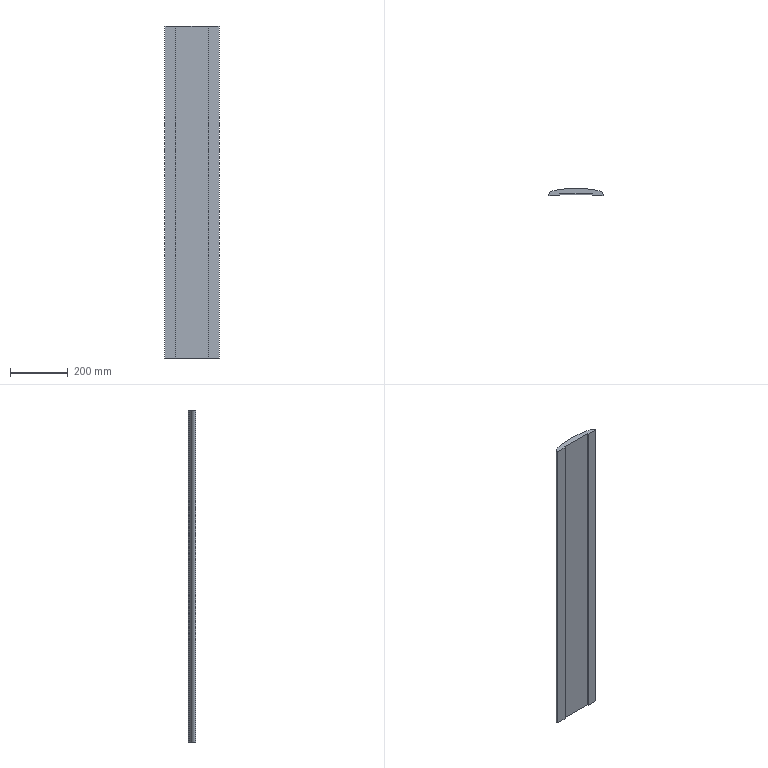Part | SolidWorks | features Extrusion 1, Fillet 1 | 1 solid | 31 faces | box 188.037 x 25 x 1150 mm | volume 3794355 mm3 | cylinder 24 | plane 7 | commonest cylinder face diameters 0.2 x8 0.6 x6 661 x5 28 x3 0.4 x2
STEP:
#1=CARTESIAN_POINT('',(-94.018,0.7177,575.));
#2=VERTEX_POINT('',#1);
#3=CARTESIAN_POINT('',(-94.012,0.2909,575.));
#4=VERTEX_POINT('',#3);
#5=CARTESIAN_POINT('',(-80.018,0.7177,575.));
#6=DIRECTION('',(0.,0.,1.));
#7=DIRECTION('',(1.,0.,0.));
#8=AXIS2_PLACEMENT_3D('',#5,#6,#7);
#9=CIRCLE('',#8,14.);
#10=EDGE_CURVE('',#2,#4,#9,.T.);
#11=ORIENTED_EDGE('',*,*,#10,.F.);
#12=CARTESIAN_POINT('',(-94.018,0.7177,-575.));
#13=VERTEX_POINT('',#12);
#14=CARTESIAN_POINT('',(-94.018,0.7177,575.));
#15=DIRECTION('',(0.,0.,-1.));
#16=VECTOR('',#15,1000.);
#17=LINE('',#14,#16);
#18=EDGE_CURVE('',#2,#13,#17,.T.);
#19=ORIENTED_EDGE('',*,*,#18,.T.);
#20=CARTESIAN_POINT('',(-94.012,0.2909,-575.));
#21=VERTEX_POINT('',#20);
#22=CARTESIAN_POINT('',(-80.018,0.7177,-575.));
#23=DIRECTION('',(0.,0.,1.));
#24=DIRECTION('',(1.,0.,0.));
#25=AXIS2_PLACEMENT_3D('',#22,#23,#24);
#26=CIRCLE('',#25,14.);
#27=EDGE_CURVE('',#13,#21,#26,.T.);
#28=ORIENTED_EDGE('',*,*,#27,.T.);
#29=CARTESIAN_POINT('',(-94.012,0.2909,575.));
#30=DIRECTION('',(0.,0.,1.));
#31=VECTOR('',#30,1000.);
#32=LINE('',#29,#31);
#33=EDGE_CURVE('',#21,#4,#32,.T.);
#34=ORIENTED_EDGE('',*,*,#33,.T.);
#35=EDGE_LOOP('',(#11,#19,#28,#34));
#36=FACE_OUTER_BOUND('',#35,.T.);
#37=CARTESIAN_POINT('',(-80.018,0.7177,575.));
#38=DIRECTION('',(0.,0.,-1.));
#39=DIRECTION('',(-1.,0.,0.));
#40=AXIS2_PLACEMENT_3D('',#37,#38,#39);
#41=CYLINDRICAL_SURFACE('',#40,14.);
#42=ADVANCED_FACE('',(#36),#41,.T.);
#43=ORIENTED_EDGE('',*,*,#18,.F.);
#44=CARTESIAN_POINT('',(-83.558,14.263,575.));
#45=VERTEX_POINT('',#44);
#46=CARTESIAN_POINT('',(-80.018,0.7177,575.));
#47=DIRECTION('',(0.,0.,1.));
#48=DIRECTION('',(1.,0.,0.));
#49=AXIS2_PLACEMENT_3D('',#46,#47,#48);
#50=CIRCLE('',#49,14.);
#51=EDGE_CURVE('',#45,#2,#50,.T.);
#52=ORIENTED_EDGE('',*,*,#51,.F.);
#53=CARTESIAN_POINT('',(-83.558,14.263,-575.));
#54=VERTEX_POINT('',#53);
#55=CARTESIAN_POINT('',(-83.558,14.263,575.));
#56=DIRECTION('',(0.,0.,-1.));
#57=VECTOR('',#56,1000.);
#58=LINE('',#55,#57);
#59=EDGE_CURVE('',#45,#54,#58,.T.);
#60=ORIENTED_EDGE('',*,*,#59,.T.);
#61=CARTESIAN_POINT('',(-80.018,0.7177,-575.));
#62=DIRECTION('',(0.,0.,1.));
#63=DIRECTION('',(1.,0.,0.));
#64=AXIS2_PLACEMENT_3D('',#61,#62,#63);
#65=CIRCLE('',#64,14.);
#66=EDGE_CURVE('',#54,#13,#65,.T.);
#67=ORIENTED_EDGE('',*,*,#66,.T.);
#68=EDGE_LOOP('',(#43,#52,#60,#67));
#69=FACE_OUTER_BOUND('',#68,.T.);
#70=CARTESIAN_POINT('',(-80.018,0.7177,575.));
#71=DIRECTION('',(0.,0.,-1.));
#72=DIRECTION('',(-1.,0.,0.));
#73=AXIS2_PLACEMENT_3D('',#70,#71,#72);
#74=CYLINDRICAL_SURFACE('',#73,14.);
#75=ADVANCED_FACE('',(#69),#74,.T.);
#76=CARTESIAN_POINT('',(-93.712,0.,575.));
#77=VERTEX_POINT('',#76);
#78=CARTESIAN_POINT('',(-56.7,0.,575.));
#79=VERTEX_POINT('',#78);
#80=CARTESIAN_POINT('',(-56.7,0.,575.));
#81=DIRECTION('',(1.,0.,0.));
#82=VECTOR('',#81,1000.);
#83=LINE('',#80,#82);
#84=EDGE_CURVE('',#77,#79,#83,.T.);
#85=ORIENTED_EDGE('',*,*,#84,.F.);
#86=CARTESIAN_POINT('',(-93.712,0.,-575.));
#87=VERTEX_POINT('',#86);
#88=CARTESIAN_POINT('',(-93.712,0.,575.));
#89=DIRECTION('',(0.,0.,-1.));
#90=VECTOR('',#89,1000.);
#91=LINE('',#88,#90);
#92=EDGE_CURVE('',#77,#87,#91,.T.);
#93=ORIENTED_EDGE('',*,*,#92,.T.);
#94=CARTESIAN_POINT('',(-56.7,0.,-575.));
#95=VERTEX_POINT('',#94);
#96=CARTESIAN_POINT('',(-56.7,0.,-575.));
#97=DIRECTION('',(1.,0.,0.));
#98=VECTOR('',#97,1000.);
#99=LINE('',#96,#98);
#100=EDGE_CURVE('',#87,#95,#99,.T.);
#101=ORIENTED_EDGE('',*,*,#100,.T.);
#102=CARTESIAN_POINT('',(-56.7,0.,575.));
#103=DIRECTION('',(0.,0.,-1.));
#104=VECTOR('',#103,1000.);
#105=LINE('',#102,#104);
#106=EDGE_CURVE('',#79,#95,#105,.T.);
#107=ORIENTED_EDGE('',*,*,#106,.F.);
#108=EDGE_LOOP('',(#85,#93,#101,#107));
#109=FACE_OUTER_BOUND('',#108,.T.);
#110=CARTESIAN_POINT('',(-56.7,0.,575.));
#111=DIRECTION('',(0.,1.,0.));
#112=DIRECTION('',(-1.,0.,0.));
#113=AXIS2_PLACEMENT_3D('',#110,#111,#112);
#114=PLANE('',#113);
#115=ADVANCED_FACE('',(#109),#114,.F.);
#116=CARTESIAN_POINT('',(-56.5,0.2,-575.));
#117=VERTEX_POINT('',#116);
#118=CARTESIAN_POINT('',(-56.7,0.2,-575.));
#119=DIRECTION('',(0.,0.,1.));
#120=DIRECTION('',(-1.,0.,0.));
#121=AXIS2_PLACEMENT_3D('',#118,#119,#120);
#122=CIRCLE('',#121,0.2);
#123=EDGE_CURVE('',#95,#117,#122,.T.);
#124=ORIENTED_EDGE('',*,*,#123,.T.);
#125=CARTESIAN_POINT('',(-56.5,0.2,575.));
#126=VERTEX_POINT('',#125);
#127=CARTESIAN_POINT('',(-56.5,0.2,575.));
#128=DIRECTION('',(0.,0.,-1.));
#129=VECTOR('',#128,1000.);
#130=LINE('',#127,#129);
#131=EDGE_CURVE('',#126,#117,#130,.T.);
#132=ORIENTED_EDGE('',*,*,#131,.F.);
#133=CARTESIAN_POINT('',(-56.7,0.2,575.));
#134=DIRECTION('',(0.,0.,1.));
#135=DIRECTION('',(-1.,0.,0.));
#136=AXIS2_PLACEMENT_3D('',#133,#134,#135);
#137=CIRCLE('',#136,0.2);
#138=EDGE_CURVE('',#79,#126,#137,.T.);
#139=ORIENTED_EDGE('',*,*,#138,.F.);
#140=ORIENTED_EDGE('',*,*,#106,.T.);
#141=EDGE_LOOP('',(#124,#132,#139,#140));
#142=FACE_OUTER_BOUND('',#141,.T.);
#143=CARTESIAN_POINT('',(-56.7,0.2,575.));
#144=DIRECTION('',(0.,0.,-1.));
#145=DIRECTION('',(-1.,0.,0.));
#146=AXIS2_PLACEMENT_3D('',#143,#144,#145);
#147=CYLINDRICAL_SURFACE('',#146,0.2);
#148=ADVANCED_FACE('',(#142),#147,.T.);
#149=CARTESIAN_POINT('',(-56.5,4.5,-575.));
#150=VERTEX_POINT('',#149);
#151=CARTESIAN_POINT('',(-56.5,0.2,-575.));
#152=DIRECTION('',(0.,1.,0.));
#153=VECTOR('',#152,1000.);
#154=LINE('',#151,#153);
#155=EDGE_CURVE('',#117,#150,#154,.T.);
#156=ORIENTED_EDGE('',*,*,#155,.T.);
#157=CARTESIAN_POINT('',(-56.5,4.5,575.));
#158=VERTEX_POINT('',#157);
#159=CARTESIAN_POINT('',(-56.5,4.5,575.));
#160=DIRECTION('',(0.,0.,-1.));
#161=VECTOR('',#160,1000.);
#162=LINE('',#159,#161);
#163=EDGE_CURVE('',#158,#150,#162,.T.);
#164=ORIENTED_EDGE('',*,*,#163,.F.);
#165=CARTESIAN_POINT('',(-56.5,0.2,575.));
#166=DIRECTION('',(0.,1.,0.));
#167=VECTOR('',#166,1000.);
#168=LINE('',#165,#167);
#169=EDGE_CURVE('',#126,#158,#168,.T.);
#170=ORIENTED_EDGE('',*,*,#169,.F.);
#171=ORIENTED_EDGE('',*,*,#131,.T.);
#172=EDGE_LOOP('',(#156,#164,#170,#171));
#173=FACE_OUTER_BOUND('',#172,.T.);
#174=CARTESIAN_POINT('',(-56.5,0.2,575.));
#175=DIRECTION('',(-1.,0.,0.));
#176=DIRECTION('',(0.,-1.,0.));
#177=AXIS2_PLACEMENT_3D('',#174,#175,#176);
#178=PLANE('',#177);
#179=ADVANCED_FACE('',(#173),#178,.F.);
#180=CARTESIAN_POINT('',(56.5,4.5,-575.));
#181=VERTEX_POINT('',#180);
#182=CARTESIAN_POINT('',(-56.5,4.5,-575.));
#183=DIRECTION('',(1.,0.,0.));
#184=VECTOR('',#183,1000.);
#185=LINE('',#182,#184);
#186=EDGE_CURVE('',#150,#181,#185,.T.);
#187=ORIENTED_EDGE('',*,*,#186,.T.);
#188=CARTESIAN_POINT('',(56.5,4.5,575.));
#189=VERTEX_POINT('',#188);
#190=CARTESIAN_POINT('',(56.5,4.5,575.));
#191=DIRECTION('',(0.,0.,-1.));
#192=VECTOR('',#191,1000.);
#193=LINE('',#190,#192);
#194=EDGE_CURVE('',#189,#181,#193,.T.);
#195=ORIENTED_EDGE('',*,*,#194,.F.);
#196=CARTESIAN_POINT('',(-56.5,4.5,575.));
#197=DIRECTION('',(1.,0.,0.));
#198=VECTOR('',#197,1000.);
#199=LINE('',#196,#198);
#200=EDGE_CURVE('',#158,#189,#199,.T.);
#201=ORIENTED_EDGE('',*,*,#200,.F.);
#202=ORIENTED_EDGE('',*,*,#163,.T.);
#203=EDGE_LOOP('',(#187,#195,#201,#202));
#204=FACE_OUTER_BOUND('',#203,.T.);
#205=CARTESIAN_POINT('',(-56.5,4.5,575.));
#206=DIRECTION('',(0.,1.,0.));
#207=DIRECTION('',(-1.,0.,0.));
#208=AXIS2_PLACEMENT_3D('',#205,#206,#207);
#209=PLANE('',#208);
#210=ADVANCED_FACE('',(#204),#209,.F.);
#211=CARTESIAN_POINT('',(56.5,0.2,-575.));
#212=VERTEX_POINT('',#211);
#213=CARTESIAN_POINT('',(56.5,0.2,-575.));
#214=DIRECTION('',(0.,-1.,0.));
#215=VECTOR('',#214,1000.);
#216=LINE('',#213,#215);
#217=EDGE_CURVE('',#181,#212,#216,.T.);
#218=ORIENTED_EDGE('',*,*,#217,.T.);
#219=CARTESIAN_POINT('',(56.5,0.2,575.));
#220=VERTEX_POINT('',#219);
#221=CARTESIAN_POINT('',(56.5,0.2,575.));
#222=DIRECTION('',(0.,0.,-1.));
#223=VECTOR('',#222,1000.);
#224=LINE('',#221,#223);
#225=EDGE_CURVE('',#220,#212,#224,.T.);
#226=ORIENTED_EDGE('',*,*,#225,.F.);
#227=CARTESIAN_POINT('',(56.5,0.2,575.));
#228=DIRECTION('',(0.,-1.,0.));
#229=VECTOR('',#228,1000.);
#230=LINE('',#227,#229);
#231=EDGE_CURVE('',#189,#220,#230,.T.);
#232=ORIENTED_EDGE('',*,*,#231,.F.);
#233=ORIENTED_EDGE('',*,*,#194,.T.);
#234=EDGE_LOOP('',(#218,#226,#232,#233));
#235=FACE_OUTER_BOUND('',#234,.T.);
#236=CARTESIAN_POINT('',(56.5,0.2,575.));
#237=DIRECTION('',(1.,0.,0.));
#238=DIRECTION('',(0.,1.,0.));
#239=AXIS2_PLACEMENT_3D('',#236,#237,#238);
#240=PLANE('',#239);
#241=ADVANCED_FACE('',(#235),#240,.F.);
#242=CARTESIAN_POINT('',(56.7,0.,-575.));
#243=VERTEX_POINT('',#242);
#244=CARTESIAN_POINT('',(56.7,0.2,-575.));
#245=DIRECTION('',(0.,0.,1.));
#246=DIRECTION('',(-1.,0.,0.));
#247=AXIS2_PLACEMENT_3D('',#244,#245,#246);
#248=CIRCLE('',#247,0.2);
#249=EDGE_CURVE('',#212,#243,#248,.T.);
#250=ORIENTED_EDGE('',*,*,#249,.T.);
#251=CARTESIAN_POINT('',(56.7,0.,575.));
#252=VERTEX_POINT('',#251);
#253=CARTESIAN_POINT('',(56.7,0.,575.));
#254=DIRECTION('',(0.,0.,-1.));
#255=VECTOR('',#254,1000.);
#256=LINE('',#253,#255);
#257=EDGE_CURVE('',#252,#243,#256,.T.);
#258=ORIENTED_EDGE('',*,*,#257,.F.);
#259=CARTESIAN_POINT('',(56.7,0.2,575.));
#260=DIRECTION('',(0.,0.,1.));
#261=DIRECTION('',(-1.,0.,0.));
#262=AXIS2_PLACEMENT_3D('',#259,#260,#261);
#263=CIRCLE('',#262,0.2);
#264=EDGE_CURVE('',#220,#252,#263,.T.);
#265=ORIENTED_EDGE('',*,*,#264,.F.);
#266=ORIENTED_EDGE('',*,*,#225,.T.);
#267=EDGE_LOOP('',(#250,#258,#265,#266));
#268=FACE_OUTER_BOUND('',#267,.T.);
#269=CARTESIAN_POINT('',(56.7,0.2,575.));
#270=DIRECTION('',(0.,0.,-1.));
#271=DIRECTION('',(-1.,0.,0.));
#272=AXIS2_PLACEMENT_3D('',#269,#270,#271);
#273=CYLINDRICAL_SURFACE('',#272,0.2);
#274=ADVANCED_FACE('',(#268),#273,.T.);
#275=CARTESIAN_POINT('',(93.712,0.,-575.));
#276=VERTEX_POINT('',#275);
#277=CARTESIAN_POINT('',(94.,0.,-575.));
#278=DIRECTION('',(1.,0.,0.));
#279=VECTOR('',#278,1000.);
#280=LINE('',#277,#279);
#281=EDGE_CURVE('',#243,#276,#280,.T.);
#282=ORIENTED_EDGE('',*,*,#281,.T.);
#283=CARTESIAN_POINT('',(93.712,0.,575.));
#284=VERTEX_POINT('',#283);
#285=CARTESIAN_POINT('',(93.712,0.,575.));
#286=DIRECTION('',(0.,0.,1.));
#287=VECTOR('',#286,1000.);
#288=LINE('',#285,#287);
#289=EDGE_CURVE('',#276,#284,#288,.T.);
#290=ORIENTED_EDGE('',*,*,#289,.T.);
#291=CARTESIAN_POINT('',(94.,0.,575.));
#292=DIRECTION('',(1.,0.,0.));
#293=VECTOR('',#292,1000.);
#294=LINE('',#291,#293);
#295=EDGE_CURVE('',#252,#284,#294,.T.);
#296=ORIENTED_EDGE('',*,*,#295,.F.);
#297=ORIENTED_EDGE('',*,*,#257,.T.);
#298=EDGE_LOOP('',(#282,#290,#296,#297));
#299=FACE_OUTER_BOUND('',#298,.T.);
#300=CARTESIAN_POINT('',(94.,0.,575.));
#301=DIRECTION('',(0.,1.,0.));
#302=DIRECTION('',(-1.,0.,0.));
#303=AXIS2_PLACEMENT_3D('',#300,#301,#302);
#304=PLANE('',#303);
#305=ADVANCED_FACE('',(#299),#304,.F.);
#306=CARTESIAN_POINT('',(94.012,0.2909,575.));
#307=VERTEX_POINT('',#306);
#308=CARTESIAN_POINT('',(83.558,14.263,575.));
#309=VERTEX_POINT('',#308);
#310=CARTESIAN_POINT('',(80.018,0.7177,575.));
#311=DIRECTION('',(0.,0.,1.));
#312=DIRECTION('',(-1.,0.,0.));
#313=AXIS2_PLACEMENT_3D('',#310,#311,#312);
#314=CIRCLE('',#313,14.);
#315=EDGE_CURVE('',#307,#309,#314,.T.);
#316=ORIENTED_EDGE('',*,*,#315,.F.);
#317=CARTESIAN_POINT('',(94.012,0.2909,-575.));
#318=VERTEX_POINT('',#317);
#319=CARTESIAN_POINT('',(94.012,0.2909,575.));
#320=DIRECTION('',(0.,0.,-1.));
#321=VECTOR('',#320,1000.);
#322=LINE('',#319,#321);
#323=EDGE_CURVE('',#307,#318,#322,.T.);
#324=ORIENTED_EDGE('',*,*,#323,.T.);
#325=CARTESIAN_POINT('',(83.558,14.263,-575.));
#326=VERTEX_POINT('',#325);
#327=CARTESIAN_POINT('',(80.018,0.7177,-575.));
#328=DIRECTION('',(0.,0.,1.));
#329=DIRECTION('',(-1.,0.,0.));
#330=AXIS2_PLACEMENT_3D('',#327,#328,#329);
#331=CIRCLE('',#330,14.);
#332=EDGE_CURVE('',#318,#326,#331,.T.);
#333=ORIENTED_EDGE('',*,*,#332,.T.);
#334=CARTESIAN_POINT('',(83.558,14.263,575.));
#335=DIRECTION('',(0.,0.,-1.));
#336=VECTOR('',#335,1000.);
#337=LINE('',#334,#336);
#338=EDGE_CURVE('',#309,#326,#337,.T.);
#339=ORIENTED_EDGE('',*,*,#338,.F.);
#340=EDGE_LOOP('',(#316,#324,#333,#339));
#341=FACE_OUTER_BOUND('',#340,.T.);
#342=CARTESIAN_POINT('',(80.018,0.7177,575.));
#343=DIRECTION('',(0.,0.,-1.));
#344=DIRECTION('',(-1.,0.,0.));
#345=AXIS2_PLACEMENT_3D('',#342,#343,#344);
#346=CYLINDRICAL_SURFACE('',#345,14.);
#347=ADVANCED_FACE('',(#341),#346,.T.);
#348=CARTESIAN_POINT('',(60.381,19.438,-575.));
#349=VERTEX_POINT('',#348);
#350=CARTESIAN_POINT('',(0.,-305.5,-575.));
#351=DIRECTION('',(0.,0.,1.));
#352=DIRECTION('',(1.,0.,0.));
#353=AXIS2_PLACEMENT_3D('',#350,#351,#352);
#354=CIRCLE('',#353,330.5);
#355=EDGE_CURVE('',#326,#349,#354,.T.);
#356=ORIENTED_EDGE('',*,*,#355,.T.);
#357=CARTESIAN_POINT('',(60.381,19.438,575.));
#358=VERTEX_POINT('',#357);
#359=CARTESIAN_POINT('',(60.381,19.438,575.));
#360=DIRECTION('',(0.,0.,-1.));
#361=VECTOR('',#360,1000.);
#362=LINE('',#359,#361);
#363=EDGE_CURVE('',#358,#349,#362,.T.);
#364=ORIENTED_EDGE('',*,*,#363,.F.);
#365=CARTESIAN_POINT('',(0.,-305.5,575.));
#366=DIRECTION('',(0.,0.,1.));
#367=DIRECTION('',(1.,0.,0.));
#368=AXIS2_PLACEMENT_3D('',#365,#366,#367);
#369=CIRCLE('',#368,330.5);
#370=EDGE_CURVE('',#309,#358,#369,.T.);
#371=ORIENTED_EDGE('',*,*,#370,.F.);
#372=ORIENTED_EDGE('',*,*,#338,.T.);
#373=EDGE_LOOP('',(#356,#364,#371,#372));
#374=FACE_OUTER_BOUND('',#373,.T.);
#375=CARTESIAN_POINT('',(0.,-305.5,575.));
#376=DIRECTION('',(0.,0.,-1.));
#377=DIRECTION('',(-1.,0.,0.));
#378=AXIS2_PLACEMENT_3D('',#375,#376,#377);
#379=CYLINDRICAL_SURFACE('',#378,330.5);
#380=ADVANCED_FACE('',(#374),#379,.T.);
#381=CARTESIAN_POINT('',(60.272,19.381,-575.));
#382=VERTEX_POINT('',#381);
#383=CARTESIAN_POINT('',(60.363,19.339,-575.));
#384=DIRECTION('',(0.,0.,1.));
#385=DIRECTION('',(1.,0.,0.));
#386=AXIS2_PLACEMENT_3D('',#383,#384,#385);
#387=CIRCLE('',#386,0.1);
#388=EDGE_CURVE('',#349,#382,#387,.T.);
#389=ORIENTED_EDGE('',*,*,#388,.T.);
#390=CARTESIAN_POINT('',(60.272,19.381,575.));
#391=VERTEX_POINT('',#390);
#392=CARTESIAN_POINT('',(60.272,19.381,575.));
#393=DIRECTION('',(0.,0.,-1.));
#394=VECTOR('',#393,1000.);
#395=LINE('',#392,#394);
#396=EDGE_CURVE('',#391,#382,#395,.T.);
#397=ORIENTED_EDGE('',*,*,#396,.F.);
#398=CARTESIAN_POINT('',(60.363,19.339,575.));
#399=DIRECTION('',(0.,0.,1.));
#400=DIRECTION('',(1.,0.,0.));
#401=AXIS2_PLACEMENT_3D('',#398,#399,#400);
#402=CIRCLE('',#401,0.1);
#403=EDGE_CURVE('',#358,#391,#402,.T.);
#404=ORIENTED_EDGE('',*,*,#403,.F.);
#405=ORIENTED_EDGE('',*,*,#363,.T.);
#406=EDGE_LOOP('',(#389,#397,#404,#405));
#407=FACE_OUTER_BOUND('',#406,.T.);
#408=CARTESIAN_POINT('',(60.363,19.339,575.));
#409=DIRECTION('',(0.,0.,-1.));
#410=DIRECTION('',(-1.,0.,0.));
#411=AXIS2_PLACEMENT_3D('',#408,#409,#410);
#412=CYLINDRICAL_SURFACE('',#411,0.1);
#413=ADVANCED_FACE('',(#407),#412,.T.);
#414=CARTESIAN_POINT('',(59.701,19.487,-575.));
#415=VERTEX_POINT('',#414);
#416=CARTESIAN_POINT('',(60.,19.508,-575.));
#417=DIRECTION('',(0.,0.,-1.));
#418=DIRECTION('',(-1.,0.,0.));
#419=AXIS2_PLACEMENT_3D('',#416,#417,#418);
#420=CIRCLE('',#419,0.3);
#421=EDGE_CURVE('',#382,#415,#420,.T.);
#422=ORIENTED_EDGE('',*,*,#421,.T.);
#423=CARTESIAN_POINT('',(59.701,19.487,575.));
#424=VERTEX_POINT('',#423);
#425=CARTESIAN_POINT('',(59.701,19.487,575.));
#426=DIRECTION('',(0.,0.,-1.));
#427=VECTOR('',#426,1000.);
#428=LINE('',#425,#427);
#429=EDGE_CURVE('',#424,#415,#428,.T.);
#430=ORIENTED_EDGE('',*,*,#429,.F.);
#431=CARTESIAN_POINT('',(60.,19.508,575.));
#432=DIRECTION('',(0.,0.,-1.));
#433=DIRECTION('',(-1.,0.,0.));
#434=AXIS2_PLACEMENT_3D('',#431,#432,#433);
#435=CIRCLE('',#434,0.3);
#436=EDGE_CURVE('',#391,#424,#435,.T.);
#437=ORIENTED_EDGE('',*,*,#436,.F.);
#438=ORIENTED_EDGE('',*,*,#396,.T.);
#439=EDGE_LOOP('',(#422,#430,#437,#438));
#440=FACE_OUTER_BOUND('',#439,.T.);
#441=CARTESIAN_POINT('',(60.,19.508,575.));
#442=DIRECTION('',(0.,0.,-1.));
#443=DIRECTION('',(-1.,0.,0.));
#444=AXIS2_PLACEMENT_3D('',#441,#442,#443);
#445=CYLINDRICAL_SURFACE('',#444,0.3);
#446=ADVANCED_FACE('',(#440),#445,.F.);
#447=CARTESIAN_POINT('',(59.619,19.578,-575.));
#448=VERTEX_POINT('',#447);
#449=CARTESIAN_POINT('',(59.601,19.48,-575.));
#450=DIRECTION('',(0.,0.,1.));
#451=DIRECTION('',(1.,0.,0.));
#452=AXIS2_PLACEMENT_3D('',#449,#450,#451);
#453=CIRCLE('',#452,0.1);
#454=EDGE_CURVE('',#415,#448,#453,.T.);
#455=ORIENTED_EDGE('',*,*,#454,.T.);
#456=CARTESIAN_POINT('',(59.619,19.578,575.));
#457=VERTEX_POINT('',#456);
#458=CARTESIAN_POINT('',(59.619,19.578,575.));
#459=DIRECTION('',(0.,0.,-1.));
#460=VECTOR('',#459,1000.);
#461=LINE('',#458,#460);
#462=EDGE_CURVE('',#457,#448,#461,.T.);
#463=ORIENTED_EDGE('',*,*,#462,.F.);
#464=CARTESIAN_POINT('',(59.601,19.48,575.));
#465=DIRECTION('',(0.,0.,1.));
#466=DIRECTION('',(1.,0.,0.));
#467=AXIS2_PLACEMENT_3D('',#464,#465,#466);
#468=CIRCLE('',#467,0.1);
#469=EDGE_CURVE('',#424,#457,#468,.T.);
#470=ORIENTED_EDGE('',*,*,#469,.F.);
#471=ORIENTED_EDGE('',*,*,#429,.T.);
#472=EDGE_LOOP('',(#455,#463,#470,#471));
#473=FACE_OUTER_BOUND('',#472,.T.);
#474=CARTESIAN_POINT('',(59.601,19.48,575.));
#475=DIRECTION('',(0.,0.,-1.));
#476=DIRECTION('',(-1.,0.,0.));
#477=AXIS2_PLACEMENT_3D('',#474,#475,#476);
#478=CYLINDRICAL_SURFACE('',#477,0.1);
#479=ADVANCED_FACE('',(#473),#478,.T.);
#480=CARTESIAN_POINT('',(59.381,19.622,-575.));
#481=VERTEX_POINT('',#480);
#482=CARTESIAN_POINT('',(0.,-305.5,-575.));
#483=DIRECTION('',(0.,0.,1.));
#484=DIRECTION('',(1.,0.,0.));
#485=AXIS2_PLACEMENT_3D('',#482,#483,#484);
#486=CIRCLE('',#485,330.5);
#487=EDGE_CURVE('',#448,#481,#486,.T.);
#488=ORIENTED_EDGE('',*,*,#487,.T.);
#489=CARTESIAN_POINT('',(59.381,19.622,575.));
#490=VERTEX_POINT('',#489);
#491=CARTESIAN_POINT('',(59.381,19.622,575.));
#492=DIRECTION('',(0.,0.,-1.));
#493=VECTOR('',#492,1000.);
#494=LINE('',#491,#493);
#495=EDGE_CURVE('',#490,#481,#494,.T.);
#496=ORIENTED_EDGE('',*,*,#495,.F.);
#497=CARTESIAN_POINT('',(0.,-305.5,575.));
#498=DIRECTION('',(0.,0.,1.));
#499=DIRECTION('',(1.,0.,0.));
#500=AXIS2_PLACEMENT_3D('',#497,#498,#499);
#501=CIRCLE('',#500,330.5);
#502=EDGE_CURVE('',#457,#490,#501,.T.);
#503=ORIENTED_EDGE('',*,*,#502,.F.);
#504=ORIENTED_EDGE('',*,*,#462,.T.);
#505=EDGE_LOOP('',(#488,#496,#503,#504));
#506=FACE_OUTER_BOUND('',#505,.T.);
#507=CARTESIAN_POINT('',(0.,-305.5,575.));
#508=DIRECTION('',(0.,0.,-1.));
#509=DIRECTION('',(-1.,0.,0.));
#510=AXIS2_PLACEMENT_3D('',#507,#508,#509);
#511=CYLINDRICAL_SURFACE('',#510,330.5);
#512=ADVANCED_FACE('',(#506),#511,.T.);
#513=CARTESIAN_POINT('',(59.272,19.565,-575.));
#514=VERTEX_POINT('',#513);
#515=CARTESIAN_POINT('',(59.363,19.523,-575.));
#516=DIRECTION('',(0.,0.,1.));
#517=DIRECTION('',(1.,0.,0.));
#518=AXIS2_PLACEMENT_3D('',#515,#516,#517);
#519=CIRCLE('',#518,0.1);
#520=EDGE_CURVE('',#481,#514,#519,.T.);
#521=ORIENTED_EDGE('',*,*,#520,.T.);
#522=CARTESIAN_POINT('',(59.272,19.565,575.));
#523=VERTEX_POINT('',#522);
#524=CARTESIAN_POINT('',(59.272,19.565,575.));
#525=DIRECTION('',(0.,0.,-1.));
#526=VECTOR('',#525,1000.);
#527=LINE('',#524,#526);
#528=EDGE_CURVE('',#523,#514,#527,.T.);
#529=ORIENTED_EDGE('',*,*,#528,.F.);
#530=CARTESIAN_POINT('',(59.363,19.523,575.));
#531=DIRECTION('',(0.,0.,1.));
#532=DIRECTION('',(1.,0.,0.));
#533=AXIS2_PLACEMENT_3D('',#530,#531,#532);
#534=CIRCLE('',#533,0.1);
#535=EDGE_CURVE('',#490,#523,#534,.T.);
#536=ORIENTED_EDGE('',*,*,#535,.F.);
#537=ORIENTED_EDGE('',*,*,#495,.T.);
#538=EDGE_LOOP('',(#521,#529,#536,#537));
#539=FACE_OUTER_BOUND('',#538,.T.);
#540=CARTESIAN_POINT('',(59.363,19.523,575.));
#541=DIRECTION('',(0.,0.,-1.));
#542=DIRECTION('',(-1.,0.,0.));
#543=AXIS2_PLACEMENT_3D('',#540,#541,#542);
#544=CYLINDRICAL_SURFACE('',#543,0.1);
#545=ADVANCED_FACE('',(#539),#544,.T.);
#546=CARTESIAN_POINT('',(58.701,19.669,-575.));
#547=VERTEX_POINT('',#546);
#548=CARTESIAN_POINT('',(59.,19.691,-575.));
#549=DIRECTION('',(0.,0.,-1.));
#550=DIRECTION('',(-1.,0.,0.));
#551=AXIS2_PLACEMENT_3D('',#548,#549,#550);
#552=CIRCLE('',#551,0.3);
#553=EDGE_CURVE('',#514,#547,#552,.T.);
#554=ORIENTED_EDGE('',*,*,#553,.T.);
#555=CARTESIAN_POINT('',(58.701,19.669,575.));
#556=VERTEX_POINT('',#555);
#557=CARTESIAN_POINT('',(58.701,19.669,575.));
#558=DIRECTION('',(0.,0.,-1.));
#559=VECTOR('',#558,1000.);
#560=LINE('',#557,#559);
#561=EDGE_CURVE('',#556,#547,#560,.T.);
#562=ORIENTED_EDGE('',*,*,#561,.F.);
#563=CARTESIAN_POINT('',(59.,19.691,575.));
#564=DIRECTION('',(0.,0.,-1.));
#565=DIRECTION('',(-1.,0.,0.));
#566=AXIS2_PLACEMENT_3D('',#563,#564,#565);
#567=CIRCLE('',#566,0.3);
#568=EDGE_CURVE('',#523,#556,#567,.T.);
#569=ORIENTED_EDGE('',*,*,#568,.F.);
#570=ORIENTED_EDGE('',*,*,#528,.T.);
#571=EDGE_LOOP('',(#554,#562,#569,#570));
#572=FACE_OUTER_BOUND('',#571,.T.);
#573=CARTESIAN_POINT('',(59.,19.691,575.));
#574=DIRECTION('',(0.,0.,-1.));
#575=DIRECTION('',(-1.,0.,0.));
#576=AXIS2_PLACEMENT_3D('',#573,#574,#575);
#577=CYLINDRICAL_SURFACE('',#576,0.3);
#578=ADVANCED_FACE('',(#572),#577,.F.);
#579=CARTESIAN_POINT('',(58.619,19.76,-575.));
#580=VERTEX_POINT('',#579);
#581=CARTESIAN_POINT('',(58.601,19.662,-575.));
#582=DIRECTION('',(0.,0.,1.));
#583=DIRECTION('',(-1.,0.,0.));
#584=AXIS2_PLACEMENT_3D('',#581,#582,#583);
#585=CIRCLE('',#584,0.1);
#586=EDGE_CURVE('',#547,#580,#585,.T.);
#587=ORIENTED_EDGE('',*,*,#586,.T.);
#588=CARTESIAN_POINT('',(58.619,19.76,575.));
#589=VERTEX_POINT('',#588);
#590=CARTESIAN_POINT('',(58.619,19.76,575.));
#591=DIRECTION('',(0.,0.,-1.));
#592=VECTOR('',#591,1000.);
#593=LINE('',#590,#592);
#594=EDGE_CURVE('',#589,#580,#593,.T.);
#595=ORIENTED_EDGE('',*,*,#594,.F.);
#596=CARTESIAN_POINT('',(58.601,19.662,575.));
#597=DIRECTION('',(0.,0.,1.));
#598=DIRECTION('',(-1.,0.,0.));
#599=AXIS2_PLACEMENT_3D('',#596,#597,#598);
#600=CIRCLE('',#599,0.1);
#601=EDGE_CURVE('',#556,#589,#600,.T.);
#602=ORIENTED_EDGE('',*,*,#601,.F.);
#603=ORIENTED_EDGE('',*,*,#561,.T.);
#604=EDGE_LOOP('',(#587,#595,#602,#603));
#605=FACE_OUTER_BOUND('',#604,.T.);
#606=CARTESIAN_POINT('',(58.601,19.662,575.));
#607=DIRECTION('',(0.,0.,-1.));
#608=DIRECTION('',(-1.,0.,0.));
#609=AXIS2_PLACEMENT_3D('',#606,#607,#608);
#610=CYLINDRICAL_SURFACE('',#609,0.1);
#611=ADVANCED_FACE('',(#605),#610,.T.);
#612=CARTESIAN_POINT('',(-58.619,19.76,-575.));
#613=VERTEX_POINT('',#612);
#614=CARTESIAN_POINT('',(0.,-305.5,-575.));
#615=DIRECTION('',(0.,0.,1.));
#616=DIRECTION('',(1.,0.,0.));
#617=AXIS2_PLACEMENT_3D('',#614,#615,#616);
#618=CIRCLE('',#617,330.5);
#619=EDGE_CURVE('',#580,#613,#618,.T.);
#620=ORIENTED_EDGE('',*,*,#619,.T.);
#621=CARTESIAN_POINT('',(-58.619,19.76,575.));
#622=VERTEX_POINT('',#621);
#623=CARTESIAN_POINT('',(-58.619,19.76,575.));
#624=DIRECTION('',(0.,0.,-1.));
#625=VECTOR('',#624,1000.);
#626=LINE('',#623,#625);
#627=EDGE_CURVE('',#622,#613,#626,.T.);
#628=ORIENTED_EDGE('',*,*,#627,.F.);
#629=CARTESIAN_POINT('',(0.,-305.5,575.));
#630=DIRECTION('',(0.,0.,1.));
#631=DIRECTION('',(1.,0.,0.));
#632=AXIS2_PLACEMENT_3D('',#629,#630,#631);
#633=CIRCLE('',#632,330.5);
#634=EDGE_CURVE('',#589,#622,#633,.T.);
#635=ORIENTED_EDGE('',*,*,#634,.F.);
#636=ORIENTED_EDGE('',*,*,#594,.T.);
#637=EDGE_LOOP('',(#620,#628,#635,#636));
#638=FACE_OUTER_BOUND('',#637,.T.);
#639=CARTESIAN_POINT('',(0.,-305.5,575.));
#640=DIRECTION('',(0.,0.,-1.));
#641=DIRECTION('',(-1.,0.,0.));
#642=AXIS2_PLACEMENT_3D('',#639,#640,#641);
#643=CYLINDRICAL_SURFACE('',#642,330.5);
#644=ADVANCED_FACE('',(#638),#643,.T.);
#645=CARTESIAN_POINT('',(-58.701,19.669,-575.));
#646=VERTEX_POINT('',#645);
#647=CARTESIAN_POINT('',(-58.601,19.662,-575.));
#648=DIRECTION('',(0.,0.,1.));
#649=DIRECTION('',(-1.,0.,0.));
#650=AXIS2_PLACEMENT_3D('',#647,#648,#649);
#651=CIRCLE('',#650,0.1);
#652=EDGE_CURVE('',#613,#646,#651,.T.);
#653=ORIENTED_EDGE('',*,*,#652,.T.);
#654=CARTESIAN_POINT('',(-58.701,19.669,575.));
#655=VERTEX_POINT('',#654);
#656=CARTESIAN_POINT('',(-58.701,19.669,575.));
#657=DIRECTION('',(0.,0.,-1.));
#658=VECTOR('',#657,1000.);
#659=LINE('',#656,#658);
#660=EDGE_CURVE('',#655,#646,#659,.T.);
#661=ORIENTED_EDGE('',*,*,#660,.F.);
#662=CARTESIAN_POINT('',(-58.601,19.662,575.));
#663=DIRECTION('',(0.,0.,1.));
#664=DIRECTION('',(-1.,0.,0.));
#665=AXIS2_PLACEMENT_3D('',#662,#663,#664);
#666=CIRCLE('',#665,0.1);
#667=EDGE_CURVE('',#622,#655,#666,.T.);
#668=ORIENTED_EDGE('',*,*,#667,.F.);
#669=ORIENTED_EDGE('',*,*,#627,.T.);
#670=EDGE_LOOP('',(#653,#661,#668,#669));
#671=FACE_OUTER_BOUND('',#670,.T.);
#672=CARTESIAN_POINT('',(-58.601,19.662,575.));
#673=DIRECTION('',(0.,0.,-1.));
#674=DIRECTION('',(-1.,0.,0.));
#675=AXIS2_PLACEMENT_3D('',#672,#673,#674);
#676=CYLINDRICAL_SURFACE('',#675,0.1);
#677=ADVANCED_FACE('',(#671),#676,.T.);
#678=CARTESIAN_POINT('',(-59.272,19.565,-575.));
#679=VERTEX_POINT('',#678);
#680=CARTESIAN_POINT('',(-59.,19.691,-575.));
#681=DIRECTION('',(0.,0.,-1.));
#682=DIRECTION('',(1.,0.,0.));
#683=AXIS2_PLACEMENT_3D('',#680,#681,#682);
#684=CIRCLE('',#683,0.3);
#685=EDGE_CURVE('',#646,#679,#684,.T.);
#686=ORIENTED_EDGE('',*,*,#685,.T.);
#687=CARTESIAN_POINT('',(-59.272,19.565,575.));
#688=VERTEX_POINT('',#687);
#689=CARTESIAN_POINT('',(-59.272,19.565,575.));
#690=DIRECTION('',(0.,0.,-1.));
#691=VECTOR('',#690,1000.);
#692=LINE('',#689,#691);
#693=EDGE_CURVE('',#688,#679,#692,.T.);
#694=ORIENTED_EDGE('',*,*,#693,.F.);
#695=CARTESIAN_POINT('',(-59.,19.691,575.));
#696=DIRECTION('',(0.,0.,-1.));
#697=DIRECTION('',(1.,0.,0.));
#698=AXIS2_PLACEMENT_3D('',#695,#696,#697);
#699=CIRCLE('',#698,0.3);
#700=EDGE_CURVE('',#655,#688,#699,.T.);
#701=ORIENTED_EDGE('',*,*,#700,.F.);
#702=ORIENTED_EDGE('',*,*,#660,.T.);
#703=EDGE_LOOP('',(#686,#694,#701,#702));
#704=FACE_OUTER_BOUND('',#703,.T.);
#705=CARTESIAN_POINT('',(-59.,19.691,575.));
#706=DIRECTION('',(0.,0.,-1.));
#707=DIRECTION('',(-1.,0.,0.));
#708=AXIS2_PLACEMENT_3D('',#705,#706,#707);
#709=CYLINDRICAL_SURFACE('',#708,0.3);
#710=ADVANCED_FACE('',(#704),#709,.F.);
#711=CARTESIAN_POINT('',(-59.381,19.622,-575.));
#712=VERTEX_POINT('',#711);
#713=CARTESIAN_POINT('',(-59.363,19.523,-575.));
#714=DIRECTION('',(0.,0.,1.));
#715=DIRECTION('',(1.,0.,0.));
#716=AXIS2_PLACEMENT_3D('',#713,#714,#715);
#717=CIRCLE('',#716,0.1);
#718=EDGE_CURVE('',#679,#712,#717,.T.);
#719=ORIENTED_EDGE('',*,*,#718,.T.);
#720=CARTESIAN_POINT('',(-59.381,19.622,575.));
#721=VERTEX_POINT('',#720);
#722=CARTESIAN_POINT('',(-59.381,19.622,575.));
#723=DIRECTION('',(0.,0.,-1.));
#724=VECTOR('',#723,1000.);
#725=LINE('',#722,#724);
#726=EDGE_CURVE('',#721,#712,#725,.T.);
#727=ORIENTED_EDGE('',*,*,#726,.F.);
#728=CARTESIAN_POINT('',(-59.363,19.523,575.));
#729=DIRECTION('',(0.,0.,1.));
#730=DIRECTION('',(1.,0.,0.));
#731=AXIS2_PLACEMENT_3D('',#728,#729,#730);
#732=CIRCLE('',#731,0.1);
#733=EDGE_CURVE('',#688,#721,#732,.T.);
#734=ORIENTED_EDGE('',*,*,#733,.F.);
#735=ORIENTED_EDGE('',*,*,#693,.T.);
#736=EDGE_LOOP('',(#719,#727,#734,#735));
#737=FACE_OUTER_BOUND('',#736,.T.);
#738=CARTESIAN_POINT('',(-59.363,19.523,575.));
#739=DIRECTION('',(0.,0.,-1.));
#740=DIRECTION('',(-1.,0.,0.));
#741=AXIS2_PLACEMENT_3D('',#738,#739,#740);
#742=CYLINDRICAL_SURFACE('',#741,0.1);
#743=ADVANCED_FACE('',(#737),#742,.T.);
#744=CARTESIAN_POINT('',(-59.619,19.578,-575.));
#745=VERTEX_POINT('',#744);
#746=CARTESIAN_POINT('',(0.,-305.5,-575.));
#747=DIRECTION('',(0.,0.,1.));
#748=DIRECTION('',(1.,0.,0.));
#749=AXIS2_PLACEMENT_3D('',#746,#747,#748);
#750=CIRCLE('',#749,330.5);
#751=EDGE_CURVE('',#712,#745,#750,.T.);
#752=ORIENTED_EDGE('',*,*,#751,.T.);
#753=CARTESIAN_POINT('',(-59.619,19.578,575.));
#754=VERTEX_POINT('',#753);
#755=CARTESIAN_POINT('',(-59.619,19.578,575.));
#756=DIRECTION('',(0.,0.,-1.));
#757=VECTOR('',#756,1000.);
#758=LINE('',#755,#757);
#759=EDGE_CURVE('',#754,#745,#758,.T.);
#760=ORIENTED_EDGE('',*,*,#759,.F.);
#761=CARTESIAN_POINT('',(0.,-305.5,575.));
#762=DIRECTION('',(0.,0.,1.));
#763=DIRECTION('',(1.,0.,0.));
#764=AXIS2_PLACEMENT_3D('',#761,#762,#763);
#765=CIRCLE('',#764,330.5);
#766=EDGE_CURVE('',#721,#754,#765,.T.);
#767=ORIENTED_EDGE('',*,*,#766,.F.);
#768=ORIENTED_EDGE('',*,*,#726,.T.);
#769=EDGE_LOOP('',(#752,#760,#767,#768));
#770=FACE_OUTER_BOUND('',#769,.T.);
#771=CARTESIAN_POINT('',(0.,-305.5,575.));
#772=DIRECTION('',(0.,0.,-1.));
#773=DIRECTION('',(-1.,0.,0.));
#774=AXIS2_PLACEMENT_3D('',#771,#772,#773);
#775=CYLINDRICAL_SURFACE('',#774,330.5);
#776=ADVANCED_FACE('',(#770),#775,.T.);
#777=CARTESIAN_POINT('',(-59.701,19.487,-575.));
#778=VERTEX_POINT('',#777);
#779=CARTESIAN_POINT('',(-59.601,19.48,-575.));
#780=DIRECTION('',(0.,0.,1.));
#781=DIRECTION('',(-1.,0.,0.));
#782=AXIS2_PLACEMENT_3D('',#779,#780,#781);
#783=CIRCLE('',#782,0.1);
#784=EDGE_CURVE('',#745,#778,#783,.T.);
#785=ORIENTED_EDGE('',*,*,#784,.T.);
#786=CARTESIAN_POINT('',(-59.701,19.487,575.));
#787=VERTEX_POINT('',#786);
#788=CARTESIAN_POINT('',(-59.701,19.487,575.));
#789=DIRECTION('',(0.,0.,-1.));
#790=VECTOR('',#789,1000.);
#791=LINE('',#788,#790);
#792=EDGE_CURVE('',#787,#778,#791,.T.);
#793=ORIENTED_EDGE('',*,*,#792,.F.);
#794=CARTESIAN_POINT('',(-59.601,19.48,575.));
#795=DIRECTION('',(0.,0.,1.));
#796=DIRECTION('',(-1.,0.,0.));
#797=AXIS2_PLACEMENT_3D('',#794,#795,#796);
#798=CIRCLE('',#797,0.1);
#799=EDGE_CURVE('',#754,#787,#798,.T.);
#800=ORIENTED_EDGE('',*,*,#799,.F.);
#801=ORIENTED_EDGE('',*,*,#759,.T.);
#802=EDGE_LOOP('',(#785,#793,#800,#801));
#803=FACE_OUTER_BOUND('',#802,.T.);
#804=CARTESIAN_POINT('',(-59.601,19.48,575.));
#805=DIRECTION('',(0.,0.,-1.));
#806=DIRECTION('',(-1.,0.,0.));
#807=AXIS2_PLACEMENT_3D('',#804,#805,#806);
#808=CYLINDRICAL_SURFACE('',#807,0.1);
#809=ADVANCED_FACE('',(#803),#808,.T.);
#810=CARTESIAN_POINT('',(-60.272,19.381,-575.));
#811=VERTEX_POINT('',#810);
#812=CARTESIAN_POINT('',(-60.,19.508,-575.));
#813=DIRECTION('',(0.,0.,-1.));
#814=DIRECTION('',(1.,0.,0.));
#815=AXIS2_PLACEMENT_3D('',#812,#813,#814);
#816=CIRCLE('',#815,0.3);
#817=EDGE_CURVE('',#778,#811,#816,.T.);
#818=ORIENTED_EDGE('',*,*,#817,.T.);
#819=CARTESIAN_POINT('',(-60.272,19.381,575.));
#820=VERTEX_POINT('',#819);
#821=CARTESIAN_POINT('',(-60.272,19.381,575.));
#822=DIRECTION('',(0.,0.,-1.));
#823=VECTOR('',#822,1000.);
#824=LINE('',#821,#823);
#825=EDGE_CURVE('',#820,#811,#824,.T.);
#826=ORIENTED_EDGE('',*,*,#825,.F.);
#827=CARTESIAN_POINT('',(-60.,19.508,575.));
#828=DIRECTION('',(0.,0.,-1.));
#829=DIRECTION('',(1.,0.,0.));
#830=AXIS2_PLACEMENT_3D('',#827,#828,#829);
#831=CIRCLE('',#830,0.3);
#832=EDGE_CURVE('',#787,#820,#831,.T.);
#833=ORIENTED_EDGE('',*,*,#832,.F.);
#834=ORIENTED_EDGE('',*,*,#792,.T.);
#835=EDGE_LOOP('',(#818,#826,#833,#834));
#836=FACE_OUTER_BOUND('',#835,.T.);
#837=CARTESIAN_POINT('',(-60.,19.508,575.));
#838=DIRECTION('',(0.,0.,-1.));
#839=DIRECTION('',(-1.,0.,0.));
#840=AXIS2_PLACEMENT_3D('',#837,#838,#839);
#841=CYLINDRICAL_SURFACE('',#840,0.3);
#842=ADVANCED_FACE('',(#836),#841,.F.);
#843=CARTESIAN_POINT('',(-60.381,19.438,-575.));
#844=VERTEX_POINT('',#843);
#845=CARTESIAN_POINT('',(-60.363,19.339,-575.));
#846=DIRECTION('',(0.,0.,1.));
#847=DIRECTION('',(1.,0.,0.));
#848=AXIS2_PLACEMENT_3D('',#845,#846,#847);
#849=CIRCLE('',#848,0.1);
#850=EDGE_CURVE('',#811,#844,#849,.T.);
#851=ORIENTED_EDGE('',*,*,#850,.T.);
#852=CARTESIAN_POINT('',(-60.381,19.438,575.));
#853=VERTEX_POINT('',#852);
#854=CARTESIAN_POINT('',(-60.381,19.438,575.));
#855=DIRECTION('',(0.,0.,-1.));
#856=VECTOR('',#855,1000.);
#857=LINE('',#854,#856);
#858=EDGE_CURVE('',#853,#844,#857,.T.);
#859=ORIENTED_EDGE('',*,*,#858,.F.);
#860=CARTESIAN_POINT('',(-60.363,19.339,575.));
#861=DIRECTION('',(0.,0.,1.));
#862=DIRECTION('',(1.,0.,0.));
#863=AXIS2_PLACEMENT_3D('',#860,#861,#862);
#864=CIRCLE('',#863,0.1);
#865=EDGE_CURVE('',#820,#853,#864,.T.);
#866=ORIENTED_EDGE('',*,*,#865,.F.);
#867=ORIENTED_EDGE('',*,*,#825,.T.);
#868=EDGE_LOOP('',(#851,#859,#866,#867));
#869=FACE_OUTER_BOUND('',#868,.T.);
#870=CARTESIAN_POINT('',(-60.363,19.339,575.));
#871=DIRECTION('',(0.,0.,-1.));
#872=DIRECTION('',(-1.,0.,0.));
#873=AXIS2_PLACEMENT_3D('',#870,#871,#872);
#874=CYLINDRICAL_SURFACE('',#873,0.1);
#875=ADVANCED_FACE('',(#869),#874,.T.);
#876=CARTESIAN_POINT('',(0.,-305.5,-575.));
#877=DIRECTION('',(0.,0.,1.));
#878=DIRECTION('',(1.,0.,0.));
#879=AXIS2_PLACEMENT_3D('',#876,#877,#878);
#880=CIRCLE('',#879,330.5);
#881=EDGE_CURVE('',#844,#54,#880,.T.);
#882=ORIENTED_EDGE('',*,*,#881,.T.);
#883=ORIENTED_EDGE('',*,*,#59,.F.);
#884=CARTESIAN_POINT('',(0.,-305.5,575.));
#885=DIRECTION('',(0.,0.,1.));
#886=DIRECTION('',(1.,0.,0.));
#887=AXIS2_PLACEMENT_3D('',#884,#885,#886);
#888=CIRCLE('',#887,330.5);
#889=EDGE_CURVE('',#853,#45,#888,.T.);
#890=ORIENTED_EDGE('',*,*,#889,.F.);
#891=ORIENTED_EDGE('',*,*,#858,.T.);
#892=EDGE_LOOP('',(#882,#883,#890,#891));
#893=FACE_OUTER_BOUND('',#892,.T.);
#894=CARTESIAN_POINT('',(0.,-305.5,575.));
#895=DIRECTION('',(0.,0.,-1.));
#896=DIRECTION('',(-1.,0.,0.));
#897=AXIS2_PLACEMENT_3D('',#894,#895,#896);
#898=CYLINDRICAL_SURFACE('',#897,330.5);
#899=ADVANCED_FACE('',(#893),#898,.T.);
#900=ORIENTED_EDGE('',*,*,#51,.T.);
#901=ORIENTED_EDGE('',*,*,#10,.T.);
#902=CARTESIAN_POINT('',(-93.712,0.3,575.));
#903=DIRECTION('',(0.,0.,1.));
#904=DIRECTION('',(1.,0.,0.));
#905=AXIS2_PLACEMENT_3D('',#902,#903,#904);
#906=CIRCLE('',#905,0.3);
#907=EDGE_CURVE('',#4,#77,#906,.T.);
#908=ORIENTED_EDGE('',*,*,#907,.T.);
#909=ORIENTED_EDGE('',*,*,#84,.T.);
#910=ORIENTED_EDGE('',*,*,#138,.T.);
#911=ORIENTED_EDGE('',*,*,#169,.T.);
#912=ORIENTED_EDGE('',*,*,#200,.T.);
#913=ORIENTED_EDGE('',*,*,#231,.T.);
#914=ORIENTED_EDGE('',*,*,#264,.T.);
#915=ORIENTED_EDGE('',*,*,#295,.T.);
#916=CARTESIAN_POINT('',(93.712,0.3,575.));
#917=DIRECTION('',(0.,0.,1.));
#918=DIRECTION('',(1.,0.,0.));
#919=AXIS2_PLACEMENT_3D('',#916,#917,#918);
#920=CIRCLE('',#919,0.3);
#921=EDGE_CURVE('',#284,#307,#920,.T.);
#922=ORIENTED_EDGE('',*,*,#921,.T.);
#923=ORIENTED_EDGE('',*,*,#315,.T.);
#924=ORIENTED_EDGE('',*,*,#370,.T.);
#925=ORIENTED_EDGE('',*,*,#403,.T.);
#926=ORIENTED_EDGE('',*,*,#436,.T.);
#927=ORIENTED_EDGE('',*,*,#469,.T.);
#928=ORIENTED_EDGE('',*,*,#502,.T.);
#929=ORIENTED_EDGE('',*,*,#535,.T.);
#930=ORIENTED_EDGE('',*,*,#568,.T.);
#931=ORIENTED_EDGE('',*,*,#601,.T.);
#932=ORIENTED_EDGE('',*,*,#634,.T.);
#933=ORIENTED_EDGE('',*,*,#667,.T.);
#934=ORIENTED_EDGE('',*,*,#700,.T.);
#935=ORIENTED_EDGE('',*,*,#733,.T.);
#936=ORIENTED_EDGE('',*,*,#766,.T.);
#937=ORIENTED_EDGE('',*,*,#799,.T.);
#938=ORIENTED_EDGE('',*,*,#832,.T.);
#939=ORIENTED_EDGE('',*,*,#865,.T.);
#940=ORIENTED_EDGE('',*,*,#889,.T.);
#941=EDGE_LOOP('',(#900,#901,#908,#909,#910,#911,#912,#913,#914,#915,#922,#923,#924,#925,#926,#927,#928,#929,#930,#931,#932,#933,#934,#935,#936,#937,#938,#939,#940));
#942=FACE_OUTER_BOUND('',#941,.T.);
#943=CARTESIAN_POINT('',(-80.018,0.7177,575.));
#944=DIRECTION('',(0.,0.,1.));
#945=DIRECTION('',(1.,0.,0.));
#946=AXIS2_PLACEMENT_3D('',#943,#944,#945);
#947=PLANE('',#946);
#948=ADVANCED_FACE('',(#942),#947,.T.);
#949=ORIENTED_EDGE('',*,*,#100,.F.);
#950=CARTESIAN_POINT('',(-93.712,0.3,-575.));
#951=DIRECTION('',(0.,0.,-1.));
#952=DIRECTION('',(1.,0.,0.));
#953=AXIS2_PLACEMENT_3D('',#950,#951,#952);
#954=CIRCLE('',#953,0.3);
#955=EDGE_CURVE('',#87,#21,#954,.T.);
#956=ORIENTED_EDGE('',*,*,#955,.T.);
#957=ORIENTED_EDGE('',*,*,#27,.F.);
#958=ORIENTED_EDGE('',*,*,#66,.F.);
#959=ORIENTED_EDGE('',*,*,#881,.F.);
#960=ORIENTED_EDGE('',*,*,#850,.F.);
#961=ORIENTED_EDGE('',*,*,#817,.F.);
#962=ORIENTED_EDGE('',*,*,#784,.F.);
#963=ORIENTED_EDGE('',*,*,#751,.F.);
#964=ORIENTED_EDGE('',*,*,#718,.F.);
#965=ORIENTED_EDGE('',*,*,#685,.F.);
#966=ORIENTED_EDGE('',*,*,#652,.F.);
#967=ORIENTED_EDGE('',*,*,#619,.F.);
#968=ORIENTED_EDGE('',*,*,#586,.F.);
#969=ORIENTED_EDGE('',*,*,#553,.F.);
#970=ORIENTED_EDGE('',*,*,#520,.F.);
#971=ORIENTED_EDGE('',*,*,#487,.F.);
#972=ORIENTED_EDGE('',*,*,#454,.F.);
#973=ORIENTED_EDGE('',*,*,#421,.F.);
#974=ORIENTED_EDGE('',*,*,#388,.F.);
#975=ORIENTED_EDGE('',*,*,#355,.F.);
#976=ORIENTED_EDGE('',*,*,#332,.F.);
#977=CARTESIAN_POINT('',(93.712,0.3,-575.));
#978=DIRECTION('',(0.,0.,-1.));
#979=DIRECTION('',(1.,0.,0.));
#980=AXIS2_PLACEMENT_3D('',#977,#978,#979);
#981=CIRCLE('',#980,0.3);
#982=EDGE_CURVE('',#318,#276,#981,.T.);
#983=ORIENTED_EDGE('',*,*,#982,.T.);
#984=ORIENTED_EDGE('',*,*,#281,.F.);
#985=ORIENTED_EDGE('',*,*,#249,.F.);
#986=ORIENTED_EDGE('',*,*,#217,.F.);
#987=ORIENTED_EDGE('',*,*,#186,.F.);
#988=ORIENTED_EDGE('',*,*,#155,.F.);
#989=ORIENTED_EDGE('',*,*,#123,.F.);
#990=EDGE_LOOP('',(#949,#956,#957,#958,#959,#960,#961,#962,#963,#964,#965,#966,#967,#968,#969,#970,#971,#972,#973,#974,#975,#976,#983,#984,#985,#986,#987,#988,#989));
#991=FACE_OUTER_BOUND('',#990,.T.);
#992=CARTESIAN_POINT('',(-80.018,0.7177,-575.));
#993=DIRECTION('',(0.,0.,1.));
#994=DIRECTION('',(1.,0.,0.));
#995=AXIS2_PLACEMENT_3D('',#992,#993,#994);
#996=PLANE('',#995);
#997=ADVANCED_FACE('',(#991),#996,.F.);
#998=ORIENTED_EDGE('',*,*,#907,.F.);
#999=ORIENTED_EDGE('',*,*,#33,.F.);
#1000=ORIENTED_EDGE('',*,*,#955,.F.);
#1001=ORIENTED_EDGE('',*,*,#92,.F.);
#1002=EDGE_LOOP('',(#998,#999,#1000,#1001));
#1003=FACE_OUTER_BOUND('',#1002,.T.);
#1004=CARTESIAN_POINT('',(-93.712,0.3,575.));
#1005=DIRECTION('',(0.,0.,-1.));
#1006=DIRECTION('',(-1.,0.,0.));
#1007=AXIS2_PLACEMENT_3D('',#1004,#1005,#1006);
#1008=CYLINDRICAL_SURFACE('',#1007,0.3);
#1009=ADVANCED_FACE('',(#1003),#1008,.T.);
#1010=ORIENTED_EDGE('',*,*,#921,.F.);
#1011=ORIENTED_EDGE('',*,*,#289,.F.);
#1012=ORIENTED_EDGE('',*,*,#982,.F.);
#1013=ORIENTED_EDGE('',*,*,#323,.F.);
#1014=EDGE_LOOP('',(#1010,#1011,#1012,#1013));
#1015=FACE_OUTER_BOUND('',#1014,.T.);
#1016=CARTESIAN_POINT('',(93.712,0.3,575.));
#1017=DIRECTION('',(0.,0.,-1.));
#1018=DIRECTION('',(-1.,0.,0.));
#1019=AXIS2_PLACEMENT_3D('',#1016,#1017,#1018);
#1020=CYLINDRICAL_SURFACE('',#1019,0.3);
#1021=ADVANCED_FACE('',(#1015),#1020,.T.);
#1022=CLOSED_SHELL('',(#42,#75,#115,#148,#179,#210,#241,#274,#305,#347,#380,#413,#446,#479,#512,#545,#578,#611,#644,#677,#710,#743,#776,#809,#842,#875,#899,#948,#997,#1009,#1021));
#1023=MANIFOLD_SOLID_BREP('',#1022);
#1024=CARTESIAN_POINT('',(0.,0.,0.));
#1025=DIRECTION('',(0.,0.,1.));
#1026=DIRECTION('',(1.,0.,0.));
#1027=AXIS2_PLACEMENT_3D('',#1024,#1025,#1026);
#1028=(LENGTH_UNIT()NAMED_UNIT(*)SI_UNIT(.MILLI.,.METRE.));
#1029=UNCERTAINTY_MEASURE_WITH_UNIT(LENGTH_MEASURE(0.00001),#1028,'','');
#1030=(NAMED_UNIT(*)PLANE_ANGLE_UNIT()SI_UNIT($,.RADIAN.));
#1031=(NAMED_UNIT(*)SI_UNIT($,.STERADIAN.)SOLID_ANGLE_UNIT());
#1032=(GEOMETRIC_REPRESENTATION_CONTEXT(3)GLOBAL_UNCERTAINTY_ASSIGNED_CONTEXT((#1029))GLOBAL_UNIT_ASSIGNED_CONTEXT((#1028,#1030,#1031))REPRESENTATION_CONTEXT('',''));
#1033=ADVANCED_BREP_SHAPE_REPRESENTATION('',(#1023,#1027),#1032);